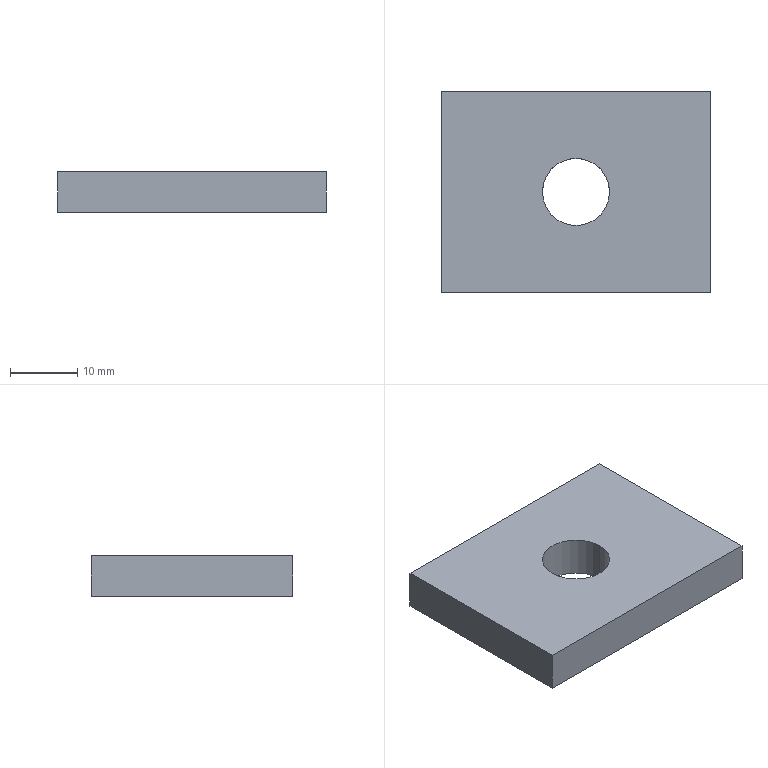Part | SolidWorks | features Extrusion 1, ICE 1 | 1 solid | 8 faces | box 40 x 30 x 6 mm | volume 6729 mm3 | plane 6 | cylinder 2 | commonest cylinder face diameters 10 x2
STEP:
#1=CARTESIAN_POINT('',(-31.669,-3.132,0.));
#2=VERTEX_POINT('',#1);
#3=CARTESIAN_POINT('',(-21.669,-3.132,0.));
#4=VERTEX_POINT('',#3);
#5=CARTESIAN_POINT('',(-26.669,-3.132,0.));
#6=DIRECTION('',(0.,0.,1.));
#7=DIRECTION('',(1.,0.,0.));
#8=AXIS2_PLACEMENT_3D('',#5,#6,#7);
#9=CIRCLE('',#8,5.);
#10=EDGE_CURVE('',#2,#4,#9,.T.);
#11=ORIENTED_EDGE('',*,*,#10,.F.);
#12=CARTESIAN_POINT('',(-31.669,-3.132,6.));
#13=VERTEX_POINT('',#12);
#14=CARTESIAN_POINT('',(-31.669,-3.132,0.));
#15=DIRECTION('',(0.,0.,1.));
#16=VECTOR('',#15,1000.);
#17=LINE('',#14,#16);
#18=EDGE_CURVE('',#2,#13,#17,.T.);
#19=ORIENTED_EDGE('',*,*,#18,.T.);
#20=CARTESIAN_POINT('',(-21.669,-3.132,6.));
#21=VERTEX_POINT('',#20);
#22=CARTESIAN_POINT('',(-26.669,-3.132,6.));
#23=DIRECTION('',(0.,0.,1.));
#24=DIRECTION('',(1.,0.,0.));
#25=AXIS2_PLACEMENT_3D('',#22,#23,#24);
#26=CIRCLE('',#25,5.);
#27=EDGE_CURVE('',#13,#21,#26,.T.);
#28=ORIENTED_EDGE('',*,*,#27,.T.);
#29=CARTESIAN_POINT('',(-21.669,-3.132,0.));
#30=DIRECTION('',(0.,0.,1.));
#31=VECTOR('',#30,1000.);
#32=LINE('',#29,#31);
#33=EDGE_CURVE('',#4,#21,#32,.T.);
#34=ORIENTED_EDGE('',*,*,#33,.F.);
#35=EDGE_LOOP('',(#11,#19,#28,#34));
#36=FACE_OUTER_BOUND('',#35,.T.);
#37=CARTESIAN_POINT('',(-26.669,-3.132,0.));
#38=DIRECTION('',(0.,0.,1.));
#39=DIRECTION('',(1.,0.,0.));
#40=AXIS2_PLACEMENT_3D('',#37,#38,#39);
#41=CYLINDRICAL_SURFACE('',#40,5.);
#42=ADVANCED_FACE('',(#36),#41,.F.);
#43=CARTESIAN_POINT('',(-46.669,11.868,0.));
#44=VERTEX_POINT('',#43);
#45=CARTESIAN_POINT('',(-46.669,-18.132,0.));
#46=VERTEX_POINT('',#45);
#47=CARTESIAN_POINT('',(-46.669,11.868,0.));
#48=DIRECTION('',(0.,-1.,0.));
#49=VECTOR('',#48,1000.);
#50=LINE('',#47,#49);
#51=EDGE_CURVE('',#44,#46,#50,.T.);
#52=ORIENTED_EDGE('',*,*,#51,.T.);
#53=CARTESIAN_POINT('',(-46.669,-18.132,6.));
#54=VERTEX_POINT('',#53);
#55=CARTESIAN_POINT('',(-46.669,-18.132,6.));
#56=DIRECTION('',(0.,0.,-1.));
#57=VECTOR('',#56,1000.);
#58=LINE('',#55,#57);
#59=EDGE_CURVE('',#54,#46,#58,.T.);
#60=ORIENTED_EDGE('',*,*,#59,.F.);
#61=CARTESIAN_POINT('',(-46.669,11.868,6.));
#62=VERTEX_POINT('',#61);
#63=CARTESIAN_POINT('',(-46.669,11.868,6.));
#64=DIRECTION('',(0.,-1.,0.));
#65=VECTOR('',#64,1000.);
#66=LINE('',#63,#65);
#67=EDGE_CURVE('',#62,#54,#66,.T.);
#68=ORIENTED_EDGE('',*,*,#67,.F.);
#69=CARTESIAN_POINT('',(-46.669,11.868,6.));
#70=DIRECTION('',(0.,0.,-1.));
#71=VECTOR('',#70,1000.);
#72=LINE('',#69,#71);
#73=EDGE_CURVE('',#62,#44,#72,.T.);
#74=ORIENTED_EDGE('',*,*,#73,.T.);
#75=EDGE_LOOP('',(#52,#60,#68,#74));
#76=FACE_OUTER_BOUND('',#75,.T.);
#77=CARTESIAN_POINT('',(-46.669,11.868,6.));
#78=DIRECTION('',(1.,0.,0.));
#79=DIRECTION('',(0.,0.,-1.));
#80=AXIS2_PLACEMENT_3D('',#77,#78,#79);
#81=PLANE('',#80);
#82=ADVANCED_FACE('',(#76),#81,.F.);
#83=CARTESIAN_POINT('',(-6.669,-18.132,0.));
#84=VERTEX_POINT('',#83);
#85=CARTESIAN_POINT('',(-46.669,-18.132,0.));
#86=DIRECTION('',(1.,0.,0.));
#87=VECTOR('',#86,1000.);
#88=LINE('',#85,#87);
#89=EDGE_CURVE('',#46,#84,#88,.T.);
#90=ORIENTED_EDGE('',*,*,#89,.T.);
#91=CARTESIAN_POINT('',(-6.669,-18.132,6.));
#92=VERTEX_POINT('',#91);
#93=CARTESIAN_POINT('',(-6.669,-18.132,6.));
#94=DIRECTION('',(0.,0.,-1.));
#95=VECTOR('',#94,1000.);
#96=LINE('',#93,#95);
#97=EDGE_CURVE('',#92,#84,#96,.T.);
#98=ORIENTED_EDGE('',*,*,#97,.F.);
#99=CARTESIAN_POINT('',(-46.669,-18.132,6.));
#100=DIRECTION('',(1.,0.,0.));
#101=VECTOR('',#100,1000.);
#102=LINE('',#99,#101);
#103=EDGE_CURVE('',#54,#92,#102,.T.);
#104=ORIENTED_EDGE('',*,*,#103,.F.);
#105=ORIENTED_EDGE('',*,*,#59,.T.);
#106=EDGE_LOOP('',(#90,#98,#104,#105));
#107=FACE_OUTER_BOUND('',#106,.T.);
#108=CARTESIAN_POINT('',(-46.669,-18.132,6.));
#109=DIRECTION('',(0.,1.,0.));
#110=DIRECTION('',(0.,0.,1.));
#111=AXIS2_PLACEMENT_3D('',#108,#109,#110);
#112=PLANE('',#111);
#113=ADVANCED_FACE('',(#107),#112,.F.);
#114=CARTESIAN_POINT('',(-6.669,11.868,0.));
#115=VERTEX_POINT('',#114);
#116=CARTESIAN_POINT('',(-6.669,11.868,0.));
#117=DIRECTION('',(0.,1.,0.));
#118=VECTOR('',#117,1000.);
#119=LINE('',#116,#118);
#120=EDGE_CURVE('',#84,#115,#119,.T.);
#121=ORIENTED_EDGE('',*,*,#120,.T.);
#122=CARTESIAN_POINT('',(-6.669,11.868,6.));
#123=VERTEX_POINT('',#122);
#124=CARTESIAN_POINT('',(-6.669,11.868,6.));
#125=DIRECTION('',(0.,0.,-1.));
#126=VECTOR('',#125,1000.);
#127=LINE('',#124,#126);
#128=EDGE_CURVE('',#123,#115,#127,.T.);
#129=ORIENTED_EDGE('',*,*,#128,.F.);
#130=CARTESIAN_POINT('',(-6.669,11.868,6.));
#131=DIRECTION('',(0.,1.,0.));
#132=VECTOR('',#131,1000.);
#133=LINE('',#130,#132);
#134=EDGE_CURVE('',#92,#123,#133,.T.);
#135=ORIENTED_EDGE('',*,*,#134,.F.);
#136=ORIENTED_EDGE('',*,*,#97,.T.);
#137=EDGE_LOOP('',(#121,#129,#135,#136));
#138=FACE_OUTER_BOUND('',#137,.T.);
#139=CARTESIAN_POINT('',(-6.669,11.868,6.));
#140=DIRECTION('',(-1.,0.,0.));
#141=DIRECTION('',(0.,-1.,0.));
#142=AXIS2_PLACEMENT_3D('',#139,#140,#141);
#143=PLANE('',#142);
#144=ADVANCED_FACE('',(#138),#143,.F.);
#145=CARTESIAN_POINT('',(-46.669,11.868,0.));
#146=DIRECTION('',(-1.,0.,0.));
#147=VECTOR('',#146,1000.);
#148=LINE('',#145,#147);
#149=EDGE_CURVE('',#115,#44,#148,.T.);
#150=ORIENTED_EDGE('',*,*,#149,.T.);
#151=ORIENTED_EDGE('',*,*,#73,.F.);
#152=CARTESIAN_POINT('',(-46.669,11.868,6.));
#153=DIRECTION('',(-1.,0.,0.));
#154=VECTOR('',#153,1000.);
#155=LINE('',#152,#154);
#156=EDGE_CURVE('',#123,#62,#155,.T.);
#157=ORIENTED_EDGE('',*,*,#156,.F.);
#158=ORIENTED_EDGE('',*,*,#128,.T.);
#159=EDGE_LOOP('',(#150,#151,#157,#158));
#160=FACE_OUTER_BOUND('',#159,.T.);
#161=CARTESIAN_POINT('',(-46.669,11.868,6.));
#162=DIRECTION('',(0.,-1.,0.));
#163=DIRECTION('',(0.,0.,-1.));
#164=AXIS2_PLACEMENT_3D('',#161,#162,#163);
#165=PLANE('',#164);
#166=ADVANCED_FACE('',(#160),#165,.F.);
#167=CARTESIAN_POINT('',(-26.669,-3.132,6.));
#168=DIRECTION('',(0.,0.,1.));
#169=DIRECTION('',(1.,0.,0.));
#170=AXIS2_PLACEMENT_3D('',#167,#168,#169);
#171=CIRCLE('',#170,5.);
#172=EDGE_CURVE('',#21,#13,#171,.T.);
#173=ORIENTED_EDGE('',*,*,#172,.F.);
#174=ORIENTED_EDGE('',*,*,#27,.F.);
#175=EDGE_LOOP('',(#173,#174));
#176=FACE_BOUND('',#175,.T.);
#177=ORIENTED_EDGE('',*,*,#67,.T.);
#178=ORIENTED_EDGE('',*,*,#103,.T.);
#179=ORIENTED_EDGE('',*,*,#134,.T.);
#180=ORIENTED_EDGE('',*,*,#156,.T.);
#181=EDGE_LOOP('',(#177,#178,#179,#180));
#182=FACE_OUTER_BOUND('',#181,.T.);
#183=CARTESIAN_POINT('',(0.,0.,6.));
#184=DIRECTION('',(0.,0.,1.));
#185=DIRECTION('',(1.,0.,0.));
#186=AXIS2_PLACEMENT_3D('',#183,#184,#185);
#187=PLANE('',#186);
#188=ADVANCED_FACE('',(#176,#182),#187,.T.);
#189=CARTESIAN_POINT('',(-26.669,-3.132,0.));
#190=DIRECTION('',(0.,0.,1.));
#191=DIRECTION('',(1.,0.,0.));
#192=AXIS2_PLACEMENT_3D('',#189,#190,#191);
#193=CIRCLE('',#192,5.);
#194=EDGE_CURVE('',#4,#2,#193,.T.);
#195=ORIENTED_EDGE('',*,*,#194,.T.);
#196=ORIENTED_EDGE('',*,*,#10,.T.);
#197=EDGE_LOOP('',(#195,#196));
#198=FACE_BOUND('',#197,.T.);
#199=ORIENTED_EDGE('',*,*,#51,.F.);
#200=ORIENTED_EDGE('',*,*,#149,.F.);
#201=ORIENTED_EDGE('',*,*,#120,.F.);
#202=ORIENTED_EDGE('',*,*,#89,.F.);
#203=EDGE_LOOP('',(#199,#200,#201,#202));
#204=FACE_OUTER_BOUND('',#203,.T.);
#205=CARTESIAN_POINT('',(0.,0.,0.));
#206=DIRECTION('',(0.,0.,1.));
#207=DIRECTION('',(1.,0.,0.));
#208=AXIS2_PLACEMENT_3D('',#205,#206,#207);
#209=PLANE('',#208);
#210=ADVANCED_FACE('',(#198,#204),#209,.F.);
#211=ORIENTED_EDGE('',*,*,#18,.F.);
#212=ORIENTED_EDGE('',*,*,#194,.F.);
#213=ORIENTED_EDGE('',*,*,#33,.T.);
#214=ORIENTED_EDGE('',*,*,#172,.T.);
#215=EDGE_LOOP('',(#211,#212,#213,#214));
#216=FACE_OUTER_BOUND('',#215,.T.);
#217=CARTESIAN_POINT('',(-26.669,-3.132,0.));
#218=DIRECTION('',(0.,0.,1.));
#219=DIRECTION('',(1.,0.,0.));
#220=AXIS2_PLACEMENT_3D('',#217,#218,#219);
#221=CYLINDRICAL_SURFACE('',#220,5.);
#222=ADVANCED_FACE('',(#216),#221,.F.);
#223=CLOSED_SHELL('',(#42,#82,#113,#144,#166,#188,#210,#222));
#224=MANIFOLD_SOLID_BREP('',#223);
#225=CARTESIAN_POINT('',(0.,0.,0.));
#226=DIRECTION('',(0.,0.,1.));
#227=DIRECTION('',(1.,0.,0.));
#228=AXIS2_PLACEMENT_3D('',#225,#226,#227);
#229=(LENGTH_UNIT()NAMED_UNIT(*)SI_UNIT(.MILLI.,.METRE.));
#230=UNCERTAINTY_MEASURE_WITH_UNIT(LENGTH_MEASURE(0.00001),#229,'','');
#231=(NAMED_UNIT(*)PLANE_ANGLE_UNIT()SI_UNIT($,.RADIAN.));
#232=(NAMED_UNIT(*)SI_UNIT($,.STERADIAN.)SOLID_ANGLE_UNIT());
#233=(GEOMETRIC_REPRESENTATION_CONTEXT(3)GLOBAL_UNCERTAINTY_ASSIGNED_CONTEXT((#230))GLOBAL_UNIT_ASSIGNED_CONTEXT((#229,#231,#232))REPRESENTATION_CONTEXT('',''));
#234=ADVANCED_BREP_SHAPE_REPRESENTATION('',(#224,#228),#233);